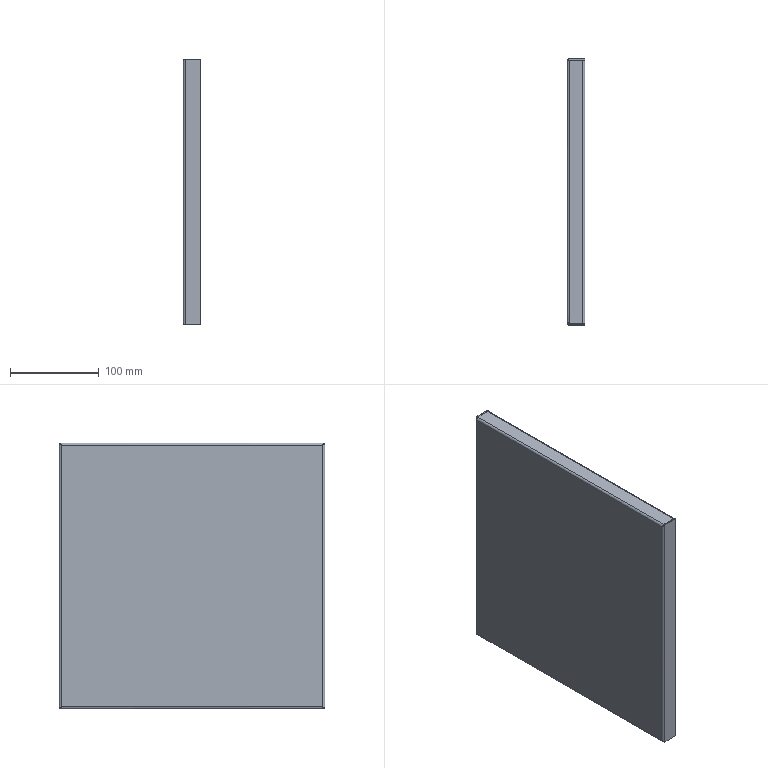Part | SolidWorks | features EdgeFlange 3, CornerFeat 1, FlatPattern 1, SMBaseFlange 1, SheetMetal 1 | 1 solid | 54 faces | box 20 x 300 x 300 mm | volume 178165 mm3 | plane 34 | cylinder 12 | spline 8 | commonest cylinder face diameters 2 x5 5 x5 1.473 x1 4.473 x1